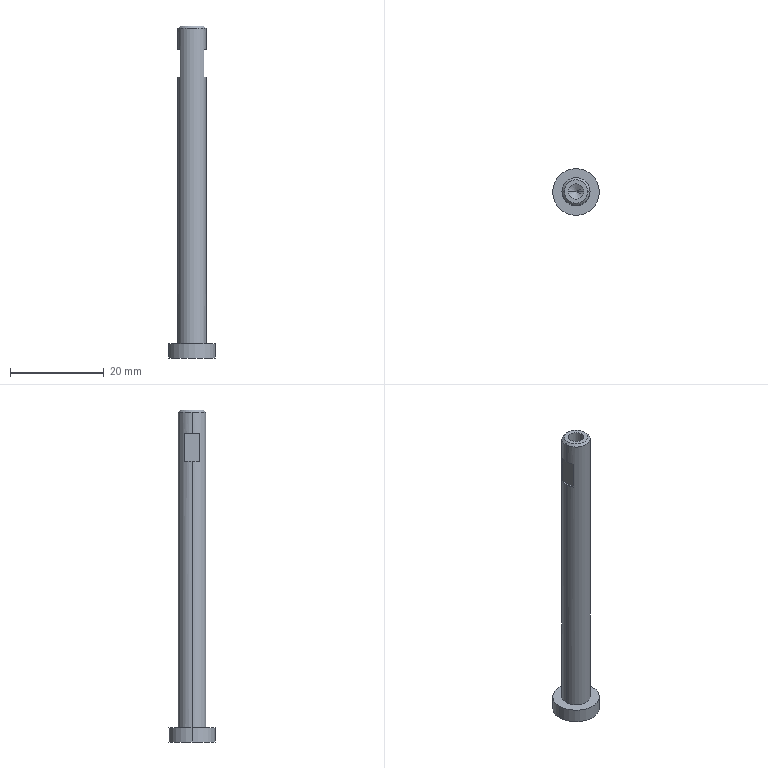Part | SolidWorks | features ICE 2, Chamfer 1, Extrusion 1, HoleWzd 1 | 1 solid | 19 faces | box 10 x 10 x 71 mm | volume 2041 mm3 | plane 9 | cylinder 6 | cone 4 | commonest cylinder face diameters 3.3 x2 6 x2 10 x2
STEP:
#1=CARTESIAN_POINT('',(-5.,0.,3.));
#2=VERTEX_POINT('',#1);
#3=CARTESIAN_POINT('',(5.,0.,3.));
#4=VERTEX_POINT('',#3);
#5=CARTESIAN_POINT('',(0.,0.,3.));
#6=DIRECTION('',(0.,0.,-1.));
#7=DIRECTION('',(-1.,0.,0.));
#8=AXIS2_PLACEMENT_3D('',#5,#6,#7);
#9=CIRCLE('',#8,5.);
#10=EDGE_CURVE('',#2,#4,#9,.T.);
#11=ORIENTED_EDGE('',*,*,#10,.T.);
#12=CARTESIAN_POINT('',(5.,0.,0.));
#13=VERTEX_POINT('',#12);
#14=CARTESIAN_POINT('',(5.,0.,3.));
#15=DIRECTION('',(0.,0.,-1.));
#16=VECTOR('',#15,1000.);
#17=LINE('',#14,#16);
#18=EDGE_CURVE('',#4,#13,#17,.T.);
#19=ORIENTED_EDGE('',*,*,#18,.T.);
#20=CARTESIAN_POINT('',(-5.,0.,0.));
#21=VERTEX_POINT('',#20);
#22=CARTESIAN_POINT('',(0.,0.,0.));
#23=DIRECTION('',(0.,0.,-1.));
#24=DIRECTION('',(-1.,0.,0.));
#25=AXIS2_PLACEMENT_3D('',#22,#23,#24);
#26=CIRCLE('',#25,5.);
#27=EDGE_CURVE('',#21,#13,#26,.T.);
#28=ORIENTED_EDGE('',*,*,#27,.F.);
#29=CARTESIAN_POINT('',(-5.,0.,3.));
#30=DIRECTION('',(0.,0.,-1.));
#31=VECTOR('',#30,1000.);
#32=LINE('',#29,#31);
#33=EDGE_CURVE('',#2,#21,#32,.T.);
#34=ORIENTED_EDGE('',*,*,#33,.F.);
#35=EDGE_LOOP('',(#11,#19,#28,#34));
#36=FACE_OUTER_BOUND('',#35,.T.);
#37=CARTESIAN_POINT('',(0.,0.,3.));
#38=DIRECTION('',(0.,0.,-1.));
#39=DIRECTION('',(-1.,0.,0.));
#40=AXIS2_PLACEMENT_3D('',#37,#38,#39);
#41=CYLINDRICAL_SURFACE('',#40,5.);
#42=ADVANCED_FACE('',(#36),#41,.T.);
#43=CARTESIAN_POINT('',(2.5,0.,71.));
#44=VERTEX_POINT('',#43);
#45=CARTESIAN_POINT('',(-2.5,0.,71.));
#46=VERTEX_POINT('',#45);
#47=CARTESIAN_POINT('',(0.,0.,71.));
#48=DIRECTION('',(0.,0.,1.));
#49=DIRECTION('',(1.,0.,0.));
#50=AXIS2_PLACEMENT_3D('',#47,#48,#49);
#51=CIRCLE('',#50,2.5);
#52=EDGE_CURVE('',#44,#46,#51,.T.);
#53=ORIENTED_EDGE('',*,*,#52,.F.);
#54=CARTESIAN_POINT('',(3.,0.,70.5));
#55=VERTEX_POINT('',#54);
#56=CARTESIAN_POINT('',(2.5,0.,71.));
#57=DIRECTION('',(0.7071,0.,-0.7071));
#58=VECTOR('',#57,1000.);
#59=LINE('',#56,#58);
#60=EDGE_CURVE('',#44,#55,#59,.T.);
#61=ORIENTED_EDGE('',*,*,#60,.T.);
#62=CARTESIAN_POINT('',(-3.,0.,70.5));
#63=VERTEX_POINT('',#62);
#64=CARTESIAN_POINT('',(0.,0.,70.5));
#65=DIRECTION('',(0.,0.,-1.));
#66=DIRECTION('',(1.,0.,0.));
#67=AXIS2_PLACEMENT_3D('',#64,#65,#66);
#68=CIRCLE('',#67,3.);
#69=EDGE_CURVE('',#63,#55,#68,.T.);
#70=ORIENTED_EDGE('',*,*,#69,.F.);
#71=CARTESIAN_POINT('',(-2.5,0.,71.));
#72=DIRECTION('',(-0.7071,0.,-0.7071));
#73=VECTOR('',#72,1000.);
#74=LINE('',#71,#73);
#75=EDGE_CURVE('',#46,#63,#74,.T.);
#76=ORIENTED_EDGE('',*,*,#75,.F.);
#77=EDGE_LOOP('',(#53,#61,#70,#76));
#78=FACE_OUTER_BOUND('',#77,.T.);
#79=CARTESIAN_POINT('',(0.,0.,71.));
#80=DIRECTION('',(0.,0.,-1.));
#81=DIRECTION('',(-1.,0.,0.));
#82=AXIS2_PLACEMENT_3D('',#79,#80,#81);
#83=CONICAL_SURFACE('',#82,2.5,0.7854);
#84=ADVANCED_FACE('',(#78),#83,.T.);
#85=CARTESIAN_POINT('',(-1.65,0.,59.5));
#86=VERTEX_POINT('',#85);
#87=CARTESIAN_POINT('',(1.65,0.,59.5));
#88=VERTEX_POINT('',#87);
#89=CARTESIAN_POINT('',(0.,0.,59.5));
#90=DIRECTION('',(0.,0.,1.));
#91=DIRECTION('',(1.,0.,0.));
#92=AXIS2_PLACEMENT_3D('',#89,#90,#91);
#93=CIRCLE('',#92,1.65);
#94=EDGE_CURVE('',#86,#88,#93,.T.);
#95=ORIENTED_EDGE('',*,*,#94,.F.);
#96=CARTESIAN_POINT('',(-1.65,0.,71.));
#97=VERTEX_POINT('',#96);
#98=CARTESIAN_POINT('',(-1.65,0.,71.));
#99=DIRECTION('',(0.,0.,1.));
#100=VECTOR('',#99,1000.);
#101=LINE('',#98,#100);
#102=EDGE_CURVE('',#86,#97,#101,.T.);
#103=ORIENTED_EDGE('',*,*,#102,.T.);
#104=CARTESIAN_POINT('',(1.65,0.,71.));
#105=VERTEX_POINT('',#104);
#106=CARTESIAN_POINT('',(0.,0.,71.));
#107=DIRECTION('',(0.,0.,1.));
#108=DIRECTION('',(1.,0.,0.));
#109=AXIS2_PLACEMENT_3D('',#106,#107,#108);
#110=CIRCLE('',#109,1.65);
#111=EDGE_CURVE('',#97,#105,#110,.T.);
#112=ORIENTED_EDGE('',*,*,#111,.T.);
#113=CARTESIAN_POINT('',(1.65,0.,71.));
#114=DIRECTION('',(0.,0.,1.));
#115=VECTOR('',#114,1000.);
#116=LINE('',#113,#115);
#117=EDGE_CURVE('',#88,#105,#116,.T.);
#118=ORIENTED_EDGE('',*,*,#117,.F.);
#119=EDGE_LOOP('',(#95,#103,#112,#118));
#120=FACE_OUTER_BOUND('',#119,.T.);
#121=CARTESIAN_POINT('',(0.,0.,71.));
#122=DIRECTION('',(0.,0.,1.));
#123=DIRECTION('',(1.,0.,0.));
#124=AXIS2_PLACEMENT_3D('',#121,#122,#123);
#125=CYLINDRICAL_SURFACE('',#124,1.65);
#126=ADVANCED_FACE('',(#120),#125,.F.);
#127=CARTESIAN_POINT('',(0.,0.,58.509));
#128=VERTEX_POINT('',#127);
#129=CARTESIAN_POINT('',(1.65,0.,59.5));
#130=DIRECTION('',(0.8572,0.,0.515));
#131=VECTOR('',#130,1000.);
#132=LINE('',#129,#131);
#133=EDGE_CURVE('',#128,#88,#132,.T.);
#134=ORIENTED_EDGE('',*,*,#133,.F.);
#135=CARTESIAN_POINT('',(-1.65,0.,59.5));
#136=DIRECTION('',(-0.8572,0.,0.515));
#137=VECTOR('',#136,1000.);
#138=LINE('',#135,#137);
#139=EDGE_CURVE('',#128,#86,#138,.T.);
#140=ORIENTED_EDGE('',*,*,#139,.T.);
#141=ORIENTED_EDGE('',*,*,#94,.T.);
#142=EDGE_LOOP('',(#134,#140,#141));
#143=FACE_OUTER_BOUND('',#142,.T.);
#144=CARTESIAN_POINT('',(0.,0.,59.5));
#145=DIRECTION('',(0.,0.,1.));
#146=DIRECTION('',(1.,0.,0.));
#147=AXIS2_PLACEMENT_3D('',#144,#145,#146);
#148=CONICAL_SURFACE('',#147,1.65,1.03);
#149=ADVANCED_FACE('',(#143),#148,.F.);
#150=ORIENTED_EDGE('',*,*,#69,.T.);
#151=CARTESIAN_POINT('',(3.,0.,66.));
#152=VERTEX_POINT('',#151);
#153=CARTESIAN_POINT('',(3.,0.,71.));
#154=DIRECTION('',(0.,0.,-1.));
#155=VECTOR('',#154,1000.);
#156=LINE('',#153,#155);
#157=EDGE_CURVE('',#55,#152,#156,.T.);
#158=ORIENTED_EDGE('',*,*,#157,.T.);
#159=CARTESIAN_POINT('',(2.5,1.658,66.));
#160=VERTEX_POINT('',#159);
#161=CARTESIAN_POINT('',(0.,0.,66.));
#162=DIRECTION('',(0.,0.,1.));
#163=DIRECTION('',(1.,0.,0.));
#164=AXIS2_PLACEMENT_3D('',#161,#162,#163);
#165=CIRCLE('',#164,3.);
#166=EDGE_CURVE('',#152,#160,#165,.T.);
#167=ORIENTED_EDGE('',*,*,#166,.T.);
#168=CARTESIAN_POINT('',(2.5,1.658,60.));
#169=VERTEX_POINT('',#168);
#170=CARTESIAN_POINT('',(2.5,1.658,71.));
#171=DIRECTION('',(0.,0.,-1.));
#172=VECTOR('',#171,1000.);
#173=LINE('',#170,#172);
#174=EDGE_CURVE('',#160,#169,#173,.T.);
#175=ORIENTED_EDGE('',*,*,#174,.T.);
#176=CARTESIAN_POINT('',(3.,0.,60.));
#177=VERTEX_POINT('',#176);
#178=CARTESIAN_POINT('',(0.,0.,60.));
#179=DIRECTION('',(0.,0.,-1.));
#180=DIRECTION('',(-1.,0.,0.));
#181=AXIS2_PLACEMENT_3D('',#178,#179,#180);
#182=CIRCLE('',#181,3.);
#183=EDGE_CURVE('',#169,#177,#182,.T.);
#184=ORIENTED_EDGE('',*,*,#183,.T.);
#185=CARTESIAN_POINT('',(3.,0.,3.));
#186=VERTEX_POINT('',#185);
#187=CARTESIAN_POINT('',(3.,0.,71.));
#188=DIRECTION('',(0.,0.,-1.));
#189=VECTOR('',#188,1000.);
#190=LINE('',#187,#189);
#191=EDGE_CURVE('',#177,#186,#190,.T.);
#192=ORIENTED_EDGE('',*,*,#191,.T.);
#193=CARTESIAN_POINT('',(-3.,0.,3.));
#194=VERTEX_POINT('',#193);
#195=CARTESIAN_POINT('',(0.,0.,3.));
#196=DIRECTION('',(0.,0.,-1.));
#197=DIRECTION('',(-1.,0.,0.));
#198=AXIS2_PLACEMENT_3D('',#195,#196,#197);
#199=CIRCLE('',#198,3.);
#200=EDGE_CURVE('',#194,#186,#199,.T.);
#201=ORIENTED_EDGE('',*,*,#200,.F.);
#202=CARTESIAN_POINT('',(-3.,0.,60.));
#203=VERTEX_POINT('',#202);
#204=CARTESIAN_POINT('',(-3.,0.,71.));
#205=DIRECTION('',(0.,0.,-1.));
#206=VECTOR('',#205,1000.);
#207=LINE('',#204,#206);
#208=EDGE_CURVE('',#203,#194,#207,.T.);
#209=ORIENTED_EDGE('',*,*,#208,.F.);
#210=CARTESIAN_POINT('',(-2.5,1.658,60.));
#211=VERTEX_POINT('',#210);
#212=CARTESIAN_POINT('',(0.,0.,60.));
#213=DIRECTION('',(0.,0.,-1.));
#214=DIRECTION('',(-1.,0.,0.));
#215=AXIS2_PLACEMENT_3D('',#212,#213,#214);
#216=CIRCLE('',#215,3.);
#217=EDGE_CURVE('',#203,#211,#216,.T.);
#218=ORIENTED_EDGE('',*,*,#217,.T.);
#219=CARTESIAN_POINT('',(-2.5,1.658,66.));
#220=VERTEX_POINT('',#219);
#221=CARTESIAN_POINT('',(-2.5,1.658,71.));
#222=DIRECTION('',(0.,0.,1.));
#223=VECTOR('',#222,1000.);
#224=LINE('',#221,#223);
#225=EDGE_CURVE('',#211,#220,#224,.T.);
#226=ORIENTED_EDGE('',*,*,#225,.T.);
#227=CARTESIAN_POINT('',(-3.,0.,66.));
#228=VERTEX_POINT('',#227);
#229=CARTESIAN_POINT('',(0.,0.,66.));
#230=DIRECTION('',(0.,0.,1.));
#231=DIRECTION('',(1.,0.,0.));
#232=AXIS2_PLACEMENT_3D('',#229,#230,#231);
#233=CIRCLE('',#232,3.);
#234=EDGE_CURVE('',#220,#228,#233,.T.);
#235=ORIENTED_EDGE('',*,*,#234,.T.);
#236=CARTESIAN_POINT('',(-3.,0.,71.));
#237=DIRECTION('',(0.,0.,-1.));
#238=VECTOR('',#237,1000.);
#239=LINE('',#236,#238);
#240=EDGE_CURVE('',#63,#228,#239,.T.);
#241=ORIENTED_EDGE('',*,*,#240,.F.);
#242=EDGE_LOOP('',(#150,#158,#167,#175,#184,#192,#201,#209,#218,#226,#235,#241));
#243=FACE_OUTER_BOUND('',#242,.T.);
#244=CARTESIAN_POINT('',(0.,0.,71.));
#245=DIRECTION('',(0.,0.,-1.));
#246=DIRECTION('',(-1.,0.,0.));
#247=AXIS2_PLACEMENT_3D('',#244,#245,#246);
#248=CYLINDRICAL_SURFACE('',#247,3.);
#249=ADVANCED_FACE('',(#243),#248,.T.);
#250=ORIENTED_EDGE('',*,*,#157,.F.);
#251=CARTESIAN_POINT('',(0.,0.,70.5));
#252=DIRECTION('',(0.,0.,-1.));
#253=DIRECTION('',(1.,0.,0.));
#254=AXIS2_PLACEMENT_3D('',#251,#252,#253);
#255=CIRCLE('',#254,3.);
#256=EDGE_CURVE('',#55,#63,#255,.T.);
#257=ORIENTED_EDGE('',*,*,#256,.T.);
#258=ORIENTED_EDGE('',*,*,#240,.T.);
#259=CARTESIAN_POINT('',(-2.5,-1.658,66.));
#260=VERTEX_POINT('',#259);
#261=CARTESIAN_POINT('',(0.,0.,66.));
#262=DIRECTION('',(0.,0.,1.));
#263=DIRECTION('',(1.,0.,0.));
#264=AXIS2_PLACEMENT_3D('',#261,#262,#263);
#265=CIRCLE('',#264,3.);
#266=EDGE_CURVE('',#228,#260,#265,.T.);
#267=ORIENTED_EDGE('',*,*,#266,.T.);
#268=CARTESIAN_POINT('',(-2.5,-1.658,60.));
#269=VERTEX_POINT('',#268);
#270=CARTESIAN_POINT('',(-2.5,-1.658,71.));
#271=DIRECTION('',(0.,0.,-1.));
#272=VECTOR('',#271,1000.);
#273=LINE('',#270,#272);
#274=EDGE_CURVE('',#260,#269,#273,.T.);
#275=ORIENTED_EDGE('',*,*,#274,.T.);
#276=CARTESIAN_POINT('',(0.,0.,60.));
#277=DIRECTION('',(0.,0.,-1.));
#278=DIRECTION('',(-1.,0.,0.));
#279=AXIS2_PLACEMENT_3D('',#276,#277,#278);
#280=CIRCLE('',#279,3.);
#281=EDGE_CURVE('',#269,#203,#280,.T.);
#282=ORIENTED_EDGE('',*,*,#281,.T.);
#283=ORIENTED_EDGE('',*,*,#208,.T.);
#284=CARTESIAN_POINT('',(0.,0.,3.));
#285=DIRECTION('',(0.,0.,-1.));
#286=DIRECTION('',(-1.,0.,0.));
#287=AXIS2_PLACEMENT_3D('',#284,#285,#286);
#288=CIRCLE('',#287,3.);
#289=EDGE_CURVE('',#186,#194,#288,.T.);
#290=ORIENTED_EDGE('',*,*,#289,.F.);
#291=ORIENTED_EDGE('',*,*,#191,.F.);
#292=CARTESIAN_POINT('',(2.5,-1.658,60.));
#293=VERTEX_POINT('',#292);
#294=CARTESIAN_POINT('',(0.,0.,60.));
#295=DIRECTION('',(0.,0.,-1.));
#296=DIRECTION('',(-1.,0.,0.));
#297=AXIS2_PLACEMENT_3D('',#294,#295,#296);
#298=CIRCLE('',#297,3.);
#299=EDGE_CURVE('',#177,#293,#298,.T.);
#300=ORIENTED_EDGE('',*,*,#299,.T.);
#301=CARTESIAN_POINT('',(2.5,-1.658,66.));
#302=VERTEX_POINT('',#301);
#303=CARTESIAN_POINT('',(2.5,-1.658,71.));
#304=DIRECTION('',(0.,0.,1.));
#305=VECTOR('',#304,1000.);
#306=LINE('',#303,#305);
#307=EDGE_CURVE('',#293,#302,#306,.T.);
#308=ORIENTED_EDGE('',*,*,#307,.T.);
#309=CARTESIAN_POINT('',(0.,0.,66.));
#310=DIRECTION('',(0.,0.,1.));
#311=DIRECTION('',(1.,0.,0.));
#312=AXIS2_PLACEMENT_3D('',#309,#310,#311);
#313=CIRCLE('',#312,3.);
#314=EDGE_CURVE('',#302,#152,#313,.T.);
#315=ORIENTED_EDGE('',*,*,#314,.T.);
#316=EDGE_LOOP('',(#250,#257,#258,#267,#275,#282,#283,#290,#291,#300,#308,#315));
#317=FACE_OUTER_BOUND('',#316,.T.);
#318=CARTESIAN_POINT('',(0.,0.,71.));
#319=DIRECTION('',(0.,0.,-1.));
#320=DIRECTION('',(-1.,0.,0.));
#321=AXIS2_PLACEMENT_3D('',#318,#319,#320);
#322=CYLINDRICAL_SURFACE('',#321,3.);
#323=ADVANCED_FACE('',(#317),#322,.T.);
#324=CARTESIAN_POINT('',(0.,0.,71.));
#325=DIRECTION('',(0.,0.,1.));
#326=DIRECTION('',(1.,0.,0.));
#327=AXIS2_PLACEMENT_3D('',#324,#325,#326);
#328=CIRCLE('',#327,2.5);
#329=EDGE_CURVE('',#46,#44,#328,.T.);
#330=ORIENTED_EDGE('',*,*,#329,.T.);
#331=ORIENTED_EDGE('',*,*,#52,.T.);
#332=EDGE_LOOP('',(#330,#331));
#333=FACE_OUTER_BOUND('',#332,.T.);
#334=CARTESIAN_POINT('',(0.,0.,71.));
#335=DIRECTION('',(0.,0.,1.));
#336=DIRECTION('',(1.,0.,0.));
#337=AXIS2_PLACEMENT_3D('',#334,#335,#336);
#338=CIRCLE('',#337,1.65);
#339=EDGE_CURVE('',#105,#97,#338,.T.);
#340=ORIENTED_EDGE('',*,*,#339,.F.);
#341=ORIENTED_EDGE('',*,*,#111,.F.);
#342=EDGE_LOOP('',(#340,#341));
#343=FACE_BOUND('',#342,.T.);
#344=CARTESIAN_POINT('',(0.,0.,71.));
#345=DIRECTION('',(0.,0.,1.));
#346=DIRECTION('',(1.,0.,0.));
#347=AXIS2_PLACEMENT_3D('',#344,#345,#346);
#348=PLANE('',#347);
#349=ADVANCED_FACE('',(#333,#343),#348,.T.);
#350=ORIENTED_EDGE('',*,*,#139,.F.);
#351=ORIENTED_EDGE('',*,*,#133,.T.);
#352=CARTESIAN_POINT('',(0.,0.,59.5));
#353=DIRECTION('',(0.,0.,1.));
#354=DIRECTION('',(1.,0.,0.));
#355=AXIS2_PLACEMENT_3D('',#352,#353,#354);
#356=CIRCLE('',#355,1.65);
#357=EDGE_CURVE('',#88,#86,#356,.T.);
#358=ORIENTED_EDGE('',*,*,#357,.T.);
#359=EDGE_LOOP('',(#350,#351,#358));
#360=FACE_OUTER_BOUND('',#359,.T.);
#361=CARTESIAN_POINT('',(0.,0.,59.5));
#362=DIRECTION('',(0.,0.,1.));
#363=DIRECTION('',(1.,0.,0.));
#364=AXIS2_PLACEMENT_3D('',#361,#362,#363);
#365=CONICAL_SURFACE('',#364,1.65,1.03);
#366=ADVANCED_FACE('',(#360),#365,.F.);
#367=ORIENTED_EDGE('',*,*,#102,.F.);
#368=ORIENTED_EDGE('',*,*,#357,.F.);
#369=ORIENTED_EDGE('',*,*,#117,.T.);
#370=ORIENTED_EDGE('',*,*,#339,.T.);
#371=EDGE_LOOP('',(#367,#368,#369,#370));
#372=FACE_OUTER_BOUND('',#371,.T.);
#373=CARTESIAN_POINT('',(0.,0.,71.));
#374=DIRECTION('',(0.,0.,1.));
#375=DIRECTION('',(1.,0.,0.));
#376=AXIS2_PLACEMENT_3D('',#373,#374,#375);
#377=CYLINDRICAL_SURFACE('',#376,1.65);
#378=ADVANCED_FACE('',(#372),#377,.F.);
#379=ORIENTED_EDGE('',*,*,#60,.F.);
#380=ORIENTED_EDGE('',*,*,#329,.F.);
#381=ORIENTED_EDGE('',*,*,#75,.T.);
#382=ORIENTED_EDGE('',*,*,#256,.F.);
#383=EDGE_LOOP('',(#379,#380,#381,#382));
#384=FACE_OUTER_BOUND('',#383,.T.);
#385=CARTESIAN_POINT('',(0.,0.,71.));
#386=DIRECTION('',(0.,0.,-1.));
#387=DIRECTION('',(-1.,0.,0.));
#388=AXIS2_PLACEMENT_3D('',#385,#386,#387);
#389=CONICAL_SURFACE('',#388,2.5,0.7854);
#390=ADVANCED_FACE('',(#384),#389,.T.);
#391=CARTESIAN_POINT('',(-2.5,-3.,60.));
#392=DIRECTION('',(0.,1.,0.));
#393=VECTOR('',#392,1000.);
#394=LINE('',#391,#393);
#395=EDGE_CURVE('',#269,#211,#394,.T.);
#396=ORIENTED_EDGE('',*,*,#395,.T.);
#397=ORIENTED_EDGE('',*,*,#217,.F.);
#398=ORIENTED_EDGE('',*,*,#281,.F.);
#399=EDGE_LOOP('',(#396,#397,#398));
#400=FACE_OUTER_BOUND('',#399,.T.);
#401=CARTESIAN_POINT('',(-5.197,-3.,60.));
#402=DIRECTION('',(0.,0.,-1.));
#403=DIRECTION('',(-1.,0.,0.));
#404=AXIS2_PLACEMENT_3D('',#401,#402,#403);
#405=PLANE('',#404);
#406=ADVANCED_FACE('',(#400),#405,.F.);
#407=CARTESIAN_POINT('',(-2.5,-3.,66.));
#408=DIRECTION('',(0.,1.,0.));
#409=VECTOR('',#408,1000.);
#410=LINE('',#407,#409);
#411=EDGE_CURVE('',#260,#220,#410,.T.);
#412=ORIENTED_EDGE('',*,*,#411,.T.);
#413=ORIENTED_EDGE('',*,*,#225,.F.);
#414=ORIENTED_EDGE('',*,*,#395,.F.);
#415=ORIENTED_EDGE('',*,*,#274,.F.);
#416=EDGE_LOOP('',(#412,#413,#414,#415));
#417=FACE_OUTER_BOUND('',#416,.T.);
#418=CARTESIAN_POINT('',(-2.5,-3.,60.));
#419=DIRECTION('',(1.,0.,0.));
#420=DIRECTION('',(0.,0.,-1.));
#421=AXIS2_PLACEMENT_3D('',#418,#419,#420);
#422=PLANE('',#421);
#423=ADVANCED_FACE('',(#417),#422,.F.);
#424=ORIENTED_EDGE('',*,*,#411,.F.);
#425=ORIENTED_EDGE('',*,*,#266,.F.);
#426=ORIENTED_EDGE('',*,*,#234,.F.);
#427=EDGE_LOOP('',(#424,#425,#426));
#428=FACE_OUTER_BOUND('',#427,.T.);
#429=CARTESIAN_POINT('',(-5.197,-3.,66.));
#430=DIRECTION('',(0.,0.,1.));
#431=DIRECTION('',(1.,0.,0.));
#432=AXIS2_PLACEMENT_3D('',#429,#430,#431);
#433=PLANE('',#432);
#434=ADVANCED_FACE('',(#428),#433,.F.);
#435=CARTESIAN_POINT('',(2.5,-3.,66.));
#436=DIRECTION('',(0.,1.,0.));
#437=VECTOR('',#436,1000.);
#438=LINE('',#435,#437);
#439=EDGE_CURVE('',#302,#160,#438,.T.);
#440=ORIENTED_EDGE('',*,*,#439,.T.);
#441=ORIENTED_EDGE('',*,*,#166,.F.);
#442=ORIENTED_EDGE('',*,*,#314,.F.);
#443=EDGE_LOOP('',(#440,#441,#442));
#444=FACE_OUTER_BOUND('',#443,.T.);
#445=CARTESIAN_POINT('',(4.862,-3.,66.));
#446=DIRECTION('',(0.,0.,1.));
#447=DIRECTION('',(1.,0.,0.));
#448=AXIS2_PLACEMENT_3D('',#445,#446,#447);
#449=PLANE('',#448);
#450=ADVANCED_FACE('',(#444),#449,.F.);
#451=ORIENTED_EDGE('',*,*,#439,.F.);
#452=ORIENTED_EDGE('',*,*,#307,.F.);
#453=CARTESIAN_POINT('',(2.5,-3.,60.));
#454=DIRECTION('',(0.,1.,0.));
#455=VECTOR('',#454,1000.);
#456=LINE('',#453,#455);
#457=EDGE_CURVE('',#293,#169,#456,.T.);
#458=ORIENTED_EDGE('',*,*,#457,.T.);
#459=ORIENTED_EDGE('',*,*,#174,.F.);
#460=EDGE_LOOP('',(#451,#452,#458,#459));
#461=FACE_OUTER_BOUND('',#460,.T.);
#462=CARTESIAN_POINT('',(2.5,-3.,60.));
#463=DIRECTION('',(-1.,0.,0.));
#464=DIRECTION('',(0.,0.,1.));
#465=AXIS2_PLACEMENT_3D('',#462,#463,#464);
#466=PLANE('',#465);
#467=ADVANCED_FACE('',(#461),#466,.F.);
#468=ORIENTED_EDGE('',*,*,#457,.F.);
#469=ORIENTED_EDGE('',*,*,#299,.F.);
#470=ORIENTED_EDGE('',*,*,#183,.F.);
#471=EDGE_LOOP('',(#468,#469,#470));
#472=FACE_OUTER_BOUND('',#471,.T.);
#473=CARTESIAN_POINT('',(4.862,-3.,60.));
#474=DIRECTION('',(0.,0.,-1.));
#475=DIRECTION('',(-1.,0.,0.));
#476=AXIS2_PLACEMENT_3D('',#473,#474,#475);
#477=PLANE('',#476);
#478=ADVANCED_FACE('',(#472),#477,.F.);
#479=ORIENTED_EDGE('',*,*,#18,.F.);
#480=CARTESIAN_POINT('',(0.,0.,3.));
#481=DIRECTION('',(0.,0.,-1.));
#482=DIRECTION('',(-1.,0.,0.));
#483=AXIS2_PLACEMENT_3D('',#480,#481,#482);
#484=CIRCLE('',#483,5.);
#485=EDGE_CURVE('',#4,#2,#484,.T.);
#486=ORIENTED_EDGE('',*,*,#485,.T.);
#487=ORIENTED_EDGE('',*,*,#33,.T.);
#488=CARTESIAN_POINT('',(0.,0.,0.));
#489=DIRECTION('',(0.,0.,-1.));
#490=DIRECTION('',(-1.,0.,0.));
#491=AXIS2_PLACEMENT_3D('',#488,#489,#490);
#492=CIRCLE('',#491,5.);
#493=EDGE_CURVE('',#13,#21,#492,.T.);
#494=ORIENTED_EDGE('',*,*,#493,.F.);
#495=EDGE_LOOP('',(#479,#486,#487,#494));
#496=FACE_OUTER_BOUND('',#495,.T.);
#497=CARTESIAN_POINT('',(0.,0.,3.));
#498=DIRECTION('',(0.,0.,-1.));
#499=DIRECTION('',(-1.,0.,0.));
#500=AXIS2_PLACEMENT_3D('',#497,#498,#499);
#501=CYLINDRICAL_SURFACE('',#500,5.);
#502=ADVANCED_FACE('',(#496),#501,.T.);
#503=ORIENTED_EDGE('',*,*,#200,.T.);
#504=ORIENTED_EDGE('',*,*,#289,.T.);
#505=EDGE_LOOP('',(#503,#504));
#506=FACE_BOUND('',#505,.T.);
#507=ORIENTED_EDGE('',*,*,#10,.F.);
#508=ORIENTED_EDGE('',*,*,#485,.F.);
#509=EDGE_LOOP('',(#507,#508));
#510=FACE_OUTER_BOUND('',#509,.T.);
#511=CARTESIAN_POINT('',(0.,0.,3.));
#512=DIRECTION('',(0.,0.,-1.));
#513=DIRECTION('',(-1.,0.,0.));
#514=AXIS2_PLACEMENT_3D('',#511,#512,#513);
#515=PLANE('',#514);
#516=ADVANCED_FACE('',(#506,#510),#515,.F.);
#517=ORIENTED_EDGE('',*,*,#27,.T.);
#518=ORIENTED_EDGE('',*,*,#493,.T.);
#519=EDGE_LOOP('',(#517,#518));
#520=FACE_OUTER_BOUND('',#519,.T.);
#521=CARTESIAN_POINT('',(0.,0.,0.));
#522=DIRECTION('',(0.,0.,1.));
#523=DIRECTION('',(1.,0.,0.));
#524=AXIS2_PLACEMENT_3D('',#521,#522,#523);
#525=PLANE('',#524);
#526=ADVANCED_FACE('',(#520),#525,.F.);
#527=CLOSED_SHELL('',(#42,#84,#126,#149,#249,#323,#349,#366,#378,#390,#406,#423,#434,#450,#467,#478,#502,#516,#526));
#528=MANIFOLD_SOLID_BREP('',#527);
#529=CARTESIAN_POINT('',(0.,0.,0.));
#530=DIRECTION('',(0.,0.,1.));
#531=DIRECTION('',(1.,0.,0.));
#532=AXIS2_PLACEMENT_3D('',#529,#530,#531);
#533=(LENGTH_UNIT()NAMED_UNIT(*)SI_UNIT(.MILLI.,.METRE.));
#534=UNCERTAINTY_MEASURE_WITH_UNIT(LENGTH_MEASURE(0.00001),#533,'','');
#535=(NAMED_UNIT(*)PLANE_ANGLE_UNIT()SI_UNIT($,.RADIAN.));
#536=(NAMED_UNIT(*)SI_UNIT($,.STERADIAN.)SOLID_ANGLE_UNIT());
#537=(GEOMETRIC_REPRESENTATION_CONTEXT(3)GLOBAL_UNCERTAINTY_ASSIGNED_CONTEXT((#534))GLOBAL_UNIT_ASSIGNED_CONTEXT((#533,#535,#536))REPRESENTATION_CONTEXT('',''));
#538=ADVANCED_BREP_SHAPE_REPRESENTATION('',(#528,#532),#537);